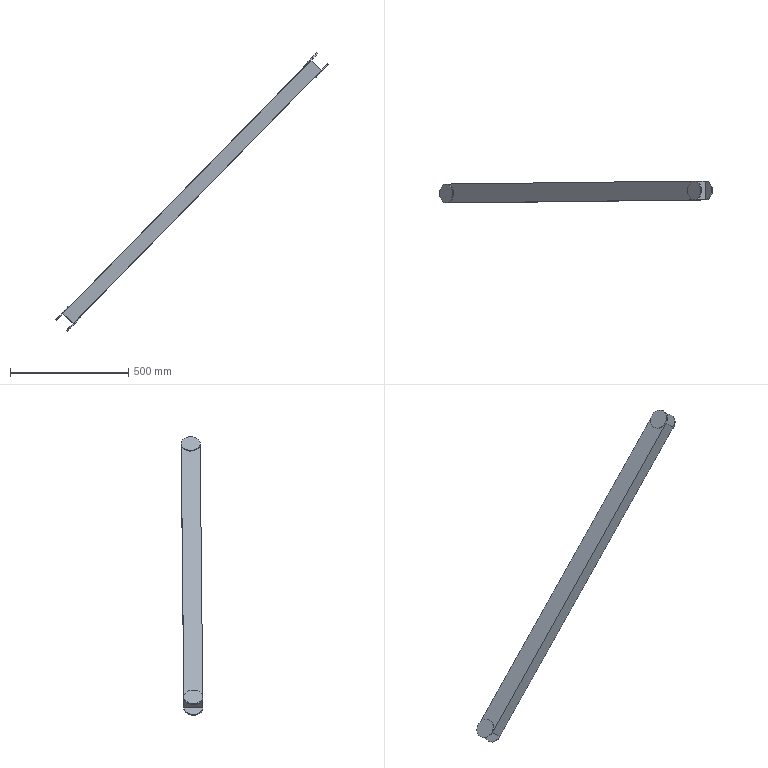Part | SolidWorks | features BaseBody 1 | 1 solid | 22 faces | box 1155 x 90.969 x 1178 mm | volume 7300531 mm3 | plane 14 | cylinder 8 | commonest cylinder face diameters 80 x8
STEP:
#1=CARTESIAN_POINT('',(-1102.13,1023.231,-2093.038));
#2=VERTEX_POINT('',#1);
#3=CARTESIAN_POINT('',(-1046.174,1023.231,-2035.863));
#4=VERTEX_POINT('',#3);
#5=CARTESIAN_POINT('',(-1074.152,1023.231,-2064.451));
#6=DIRECTION('',(0.7147,0.,-0.6994));
#7=DIRECTION('',(-0.6994,0.,-0.7147));
#8=AXIS2_PLACEMENT_3D('',#5,#6,#7);
#9=CIRCLE('',#8,40.);
#10=EDGE_CURVE('',#2,#4,#9,.T.);
#11=ORIENTED_EDGE('',*,*,#10,.T.);
#12=CARTESIAN_POINT('',(-1042.601,1023.231,-2039.36));
#13=VERTEX_POINT('',#12);
#14=CARTESIAN_POINT('',(-1046.174,1023.231,-2035.863));
#15=DIRECTION('',(0.7147,0.,-0.6994));
#16=VECTOR('',#15,1000.);
#17=LINE('',#14,#16);
#18=EDGE_CURVE('',#4,#13,#17,.T.);
#19=ORIENTED_EDGE('',*,*,#18,.T.);
#20=CARTESIAN_POINT('',(-1070.783,1063.23,-2068.157));
#21=VERTEX_POINT('',#20);
#22=CARTESIAN_POINT('',(-1070.579,1023.231,-2067.948));
#23=DIRECTION('',(-0.7147,0.,0.6994));
#24=DIRECTION('',(-0.6994,0.,-0.7147));
#25=AXIS2_PLACEMENT_3D('',#22,#23,#24);
#26=CIRCLE('',#25,40.);
#27=EDGE_CURVE('',#13,#21,#26,.T.);
#28=ORIENTED_EDGE('',*,*,#27,.T.);
#29=CARTESIAN_POINT('',(-1098.556,1023.231,-2096.535));
#30=VERTEX_POINT('',#29);
#31=CARTESIAN_POINT('',(-1070.579,1023.231,-2067.948));
#32=DIRECTION('',(-0.7147,0.,0.6994));
#33=DIRECTION('',(-0.6994,0.,-0.7147));
#34=AXIS2_PLACEMENT_3D('',#31,#32,#33);
#35=CIRCLE('',#34,40.);
#36=EDGE_CURVE('',#21,#30,#35,.T.);
#37=ORIENTED_EDGE('',*,*,#36,.T.);
#38=CARTESIAN_POINT('',(-1102.13,1023.231,-2093.038));
#39=DIRECTION('',(0.7147,0.,-0.6994));
#40=VECTOR('',#39,1000.);
#41=LINE('',#38,#40);
#42=EDGE_CURVE('',#2,#30,#41,.T.);
#43=ORIENTED_EDGE('',*,*,#42,.F.);
#44=EDGE_LOOP('',(#11,#19,#28,#37,#43));
#45=FACE_OUTER_BOUND('',#44,.T.);
#46=CARTESIAN_POINT('',(-1074.152,1023.231,-2064.451));
#47=DIRECTION('',(0.7147,0.,-0.6994));
#48=DIRECTION('',(-0.6994,0.,-0.7147));
#49=AXIS2_PLACEMENT_3D('',#46,#47,#48);
#50=CYLINDRICAL_SURFACE('',#49,40.);
#51=ADVANCED_FACE('',(#45),#50,.T.);
#52=CARTESIAN_POINT('',(-52.992,1034.2,-1021.036));
#53=VERTEX_POINT('',#52);
#54=CARTESIAN_POINT('',(2.964,1034.2,-963.861));
#55=VERTEX_POINT('',#54);
#56=CARTESIAN_POINT('',(-25.014,1034.2,-992.448));
#57=DIRECTION('',(0.7147,0.,-0.6994));
#58=DIRECTION('',(-0.6994,0.,-0.7147));
#59=AXIS2_PLACEMENT_3D('',#56,#57,#58);
#60=CIRCLE('',#59,40.);
#61=EDGE_CURVE('',#53,#55,#60,.T.);
#62=ORIENTED_EDGE('',*,*,#61,.T.);
#63=CARTESIAN_POINT('',(6.537,1034.2,-967.358));
#64=VERTEX_POINT('',#63);
#65=CARTESIAN_POINT('',(2.964,1034.2,-963.861));
#66=DIRECTION('',(0.7147,0.,-0.6994));
#67=VECTOR('',#66,1000.);
#68=LINE('',#65,#67);
#69=EDGE_CURVE('',#55,#64,#68,.T.);
#70=ORIENTED_EDGE('',*,*,#69,.T.);
#71=CARTESIAN_POINT('',(-21.645,1074.199,-996.154));
#72=VERTEX_POINT('',#71);
#73=CARTESIAN_POINT('',(-21.441,1034.2,-995.945));
#74=DIRECTION('',(-0.7147,0.,0.6994));
#75=DIRECTION('',(-0.6994,0.,-0.7147));
#76=AXIS2_PLACEMENT_3D('',#73,#74,#75);
#77=CIRCLE('',#76,40.);
#78=EDGE_CURVE('',#64,#72,#77,.T.);
#79=ORIENTED_EDGE('',*,*,#78,.T.);
#80=CARTESIAN_POINT('',(-49.418,1034.2,-1024.533));
#81=VERTEX_POINT('',#80);
#82=CARTESIAN_POINT('',(-21.441,1034.2,-995.945));
#83=DIRECTION('',(-0.7147,0.,0.6994));
#84=DIRECTION('',(-0.6994,0.,-0.7147));
#85=AXIS2_PLACEMENT_3D('',#82,#83,#84);
#86=CIRCLE('',#85,40.);
#87=EDGE_CURVE('',#72,#81,#86,.T.);
#88=ORIENTED_EDGE('',*,*,#87,.T.);
#89=CARTESIAN_POINT('',(-52.992,1034.2,-1021.036));
#90=DIRECTION('',(0.7147,0.,-0.6994));
#91=VECTOR('',#90,1000.);
#92=LINE('',#89,#91);
#93=EDGE_CURVE('',#53,#81,#92,.T.);
#94=ORIENTED_EDGE('',*,*,#93,.F.);
#95=EDGE_LOOP('',(#62,#70,#79,#88,#94));
#96=FACE_OUTER_BOUND('',#95,.T.);
#97=CARTESIAN_POINT('',(-25.014,1034.2,-992.448));
#98=DIRECTION('',(0.7147,0.,-0.6994));
#99=DIRECTION('',(-0.6994,0.,-0.7147));
#100=AXIS2_PLACEMENT_3D('',#97,#98,#99);
#101=CYLINDRICAL_SURFACE('',#100,40.);
#102=ADVANCED_FACE('',(#96),#101,.T.);
#103=CARTESIAN_POINT('',(-996.146,1023.231,-2084.824));
#104=VERTEX_POINT('',#103);
#105=CARTESIAN_POINT('',(-1052.102,1023.231,-2141.999));
#106=VERTEX_POINT('',#105);
#107=CARTESIAN_POINT('',(-1024.124,1023.231,-2113.412));
#108=DIRECTION('',(-0.7147,0.,0.6994));
#109=DIRECTION('',(0.6994,0.,0.7147));
#110=AXIS2_PLACEMENT_3D('',#107,#108,#109);
#111=CIRCLE('',#110,40.);
#112=EDGE_CURVE('',#104,#106,#111,.T.);
#113=ORIENTED_EDGE('',*,*,#112,.T.);
#114=CARTESIAN_POINT('',(-1055.675,1023.231,-2138.502));
#115=VERTEX_POINT('',#114);
#116=CARTESIAN_POINT('',(-1052.102,1023.231,-2141.999));
#117=DIRECTION('',(-0.7147,0.,0.6994));
#118=VECTOR('',#117,1000.);
#119=LINE('',#116,#118);
#120=EDGE_CURVE('',#106,#115,#119,.T.);
#121=ORIENTED_EDGE('',*,*,#120,.T.);
#122=CARTESIAN_POINT('',(-1027.902,1063.23,-2110.124));
#123=VERTEX_POINT('',#122);
#124=CARTESIAN_POINT('',(-1027.697,1023.231,-2109.915));
#125=DIRECTION('',(0.7147,0.,-0.6994));
#126=DIRECTION('',(0.6994,0.,0.7147));
#127=AXIS2_PLACEMENT_3D('',#124,#125,#126);
#128=CIRCLE('',#127,40.);
#129=EDGE_CURVE('',#115,#123,#128,.T.);
#130=ORIENTED_EDGE('',*,*,#129,.T.);
#131=CARTESIAN_POINT('',(-999.72,1023.231,-2081.327));
#132=VERTEX_POINT('',#131);
#133=CARTESIAN_POINT('',(-1027.697,1023.231,-2109.915));
#134=DIRECTION('',(0.7147,0.,-0.6994));
#135=DIRECTION('',(0.6994,0.,0.7147));
#136=AXIS2_PLACEMENT_3D('',#133,#134,#135);
#137=CIRCLE('',#136,40.);
#138=EDGE_CURVE('',#123,#132,#137,.T.);
#139=ORIENTED_EDGE('',*,*,#138,.T.);
#140=CARTESIAN_POINT('',(-996.146,1023.231,-2084.824));
#141=DIRECTION('',(-0.7147,0.,0.6994));
#142=VECTOR('',#141,1000.);
#143=LINE('',#140,#142);
#144=EDGE_CURVE('',#104,#132,#143,.T.);
#145=ORIENTED_EDGE('',*,*,#144,.F.);
#146=EDGE_LOOP('',(#113,#121,#130,#139,#145));
#147=FACE_OUTER_BOUND('',#146,.T.);
#148=CARTESIAN_POINT('',(-1024.124,1023.231,-2113.412));
#149=DIRECTION('',(-0.7147,0.,0.6994));
#150=DIRECTION('',(0.6994,0.,0.7147));
#151=AXIS2_PLACEMENT_3D('',#148,#149,#150);
#152=CYLINDRICAL_SURFACE('',#151,40.);
#153=ADVANCED_FACE('',(#147),#152,.T.);
#154=CARTESIAN_POINT('',(52.992,1034.2,-1012.822));
#155=VERTEX_POINT('',#154);
#156=CARTESIAN_POINT('',(-2.964,1034.2,-1069.997));
#157=VERTEX_POINT('',#156);
#158=CARTESIAN_POINT('',(25.014,1034.2,-1041.409));
#159=DIRECTION('',(-0.7147,0.,0.6994));
#160=DIRECTION('',(0.6994,0.,0.7147));
#161=AXIS2_PLACEMENT_3D('',#158,#159,#160);
#162=CIRCLE('',#161,40.);
#163=EDGE_CURVE('',#155,#157,#162,.T.);
#164=ORIENTED_EDGE('',*,*,#163,.T.);
#165=CARTESIAN_POINT('',(-6.537,1034.2,-1066.5));
#166=VERTEX_POINT('',#165);
#167=CARTESIAN_POINT('',(-2.964,1034.2,-1069.997));
#168=DIRECTION('',(-0.7147,0.,0.6994));
#169=VECTOR('',#168,1000.);
#170=LINE('',#167,#169);
#171=EDGE_CURVE('',#157,#166,#170,.T.);
#172=ORIENTED_EDGE('',*,*,#171,.T.);
#173=CARTESIAN_POINT('',(21.236,1074.199,-1038.121));
#174=VERTEX_POINT('',#173);
#175=CARTESIAN_POINT('',(21.441,1034.2,-1037.912));
#176=DIRECTION('',(0.7147,0.,-0.6994));
#177=DIRECTION('',(0.6994,0.,0.7147));
#178=AXIS2_PLACEMENT_3D('',#175,#176,#177);
#179=CIRCLE('',#178,40.);
#180=EDGE_CURVE('',#166,#174,#179,.T.);
#181=ORIENTED_EDGE('',*,*,#180,.T.);
#182=CARTESIAN_POINT('',(49.418,1034.2,-1009.325));
#183=VERTEX_POINT('',#182);
#184=CARTESIAN_POINT('',(21.441,1034.2,-1037.912));
#185=DIRECTION('',(0.7147,0.,-0.6994));
#186=DIRECTION('',(0.6994,0.,0.7147));
#187=AXIS2_PLACEMENT_3D('',#184,#185,#186);
#188=CIRCLE('',#187,40.);
#189=EDGE_CURVE('',#174,#183,#188,.T.);
#190=ORIENTED_EDGE('',*,*,#189,.T.);
#191=CARTESIAN_POINT('',(52.992,1034.2,-1012.822));
#192=DIRECTION('',(-0.7147,0.,0.6994));
#193=VECTOR('',#192,1000.);
#194=LINE('',#191,#193);
#195=EDGE_CURVE('',#155,#183,#194,.T.);
#196=ORIENTED_EDGE('',*,*,#195,.F.);
#197=EDGE_LOOP('',(#164,#172,#181,#190,#196));
#198=FACE_OUTER_BOUND('',#197,.T.);
#199=CARTESIAN_POINT('',(25.014,1034.2,-1041.409));
#200=DIRECTION('',(-0.7147,0.,0.6994));
#201=DIRECTION('',(0.6994,0.,0.7147));
#202=AXIS2_PLACEMENT_3D('',#199,#200,#201);
#203=CYLINDRICAL_SURFACE('',#202,40.);
#204=ADVANCED_FACE('',(#198),#203,.T.);
#205=CARTESIAN_POINT('',(-21.236,994.201,-995.736));
#206=VERTEX_POINT('',#205);
#207=CARTESIAN_POINT('',(-1070.374,983.232,-2067.739));
#208=VERTEX_POINT('',#207);
#209=CARTESIAN_POINT('',(-21.236,994.201,-995.736));
#210=DIRECTION('',(-0.6994,-0.007312,-0.7147));
#211=VECTOR('',#210,1000.);
#212=LINE('',#209,#211);
#213=EDGE_CURVE('',#206,#208,#212,.T.);
#214=ORIENTED_EDGE('',*,*,#213,.F.);
#215=CARTESIAN_POINT('',(-21.441,1034.2,-995.945));
#216=DIRECTION('',(-0.7147,0.,0.6994));
#217=DIRECTION('',(-0.6994,0.,-0.7147));
#218=AXIS2_PLACEMENT_3D('',#215,#216,#217);
#219=CIRCLE('',#218,40.);
#220=EDGE_CURVE('',#81,#206,#219,.T.);
#221=ORIENTED_EDGE('',*,*,#220,.F.);
#222=ORIENTED_EDGE('',*,*,#87,.F.);
#223=CARTESIAN_POINT('',(-1070.783,1063.23,-2068.157));
#224=DIRECTION('',(0.6994,0.007312,0.7147));
#225=VECTOR('',#224,1000.);
#226=LINE('',#223,#225);
#227=EDGE_CURVE('',#21,#72,#226,.T.);
#228=ORIENTED_EDGE('',*,*,#227,.F.);
#229=ORIENTED_EDGE('',*,*,#27,.F.);
#230=CARTESIAN_POINT('',(-1070.579,1023.231,-2067.948));
#231=DIRECTION('',(-0.7147,0.,0.6994));
#232=DIRECTION('',(-0.6994,0.,-0.7147));
#233=AXIS2_PLACEMENT_3D('',#230,#231,#232);
#234=CIRCLE('',#233,40.);
#235=EDGE_CURVE('',#208,#13,#234,.T.);
#236=ORIENTED_EDGE('',*,*,#235,.F.);
#237=EDGE_LOOP('',(#214,#221,#222,#228,#229,#236));
#238=FACE_OUTER_BOUND('',#237,.T.);
#239=CARTESIAN_POINT('',(-1070.374,983.232,-2067.739));
#240=DIRECTION('',(0.7147,0.,-0.6994));
#241=DIRECTION('',(-0.6994,0.,-0.7147));
#242=AXIS2_PLACEMENT_3D('',#239,#240,#241);
#243=PLANE('',#242);
#244=ADVANCED_FACE('',(#238),#243,.F.);
#245=ORIENTED_EDGE('',*,*,#18,.F.);
#246=CARTESIAN_POINT('',(-1074.152,1023.231,-2064.451));
#247=DIRECTION('',(0.7147,0.,-0.6994));
#248=DIRECTION('',(-0.6994,0.,-0.7147));
#249=AXIS2_PLACEMENT_3D('',#246,#247,#248);
#250=CIRCLE('',#249,40.);
#251=EDGE_CURVE('',#4,#2,#250,.T.);
#252=ORIENTED_EDGE('',*,*,#251,.T.);
#253=ORIENTED_EDGE('',*,*,#42,.T.);
#254=CARTESIAN_POINT('',(-1070.579,1023.231,-2067.948));
#255=DIRECTION('',(-0.7147,0.,0.6994));
#256=DIRECTION('',(-0.6994,0.,-0.7147));
#257=AXIS2_PLACEMENT_3D('',#254,#255,#256);
#258=CIRCLE('',#257,40.);
#259=EDGE_CURVE('',#30,#208,#258,.T.);
#260=ORIENTED_EDGE('',*,*,#259,.T.);
#261=ORIENTED_EDGE('',*,*,#235,.T.);
#262=EDGE_LOOP('',(#245,#252,#253,#260,#261));
#263=FACE_OUTER_BOUND('',#262,.T.);
#264=CARTESIAN_POINT('',(-1074.152,1023.231,-2064.451));
#265=DIRECTION('',(0.7147,0.,-0.6994));
#266=DIRECTION('',(-0.6994,0.,-0.7147));
#267=AXIS2_PLACEMENT_3D('',#264,#265,#266);
#268=CYLINDRICAL_SURFACE('',#267,40.);
#269=ADVANCED_FACE('',(#263),#268,.T.);
#270=ORIENTED_EDGE('',*,*,#213,.T.);
#271=CARTESIAN_POINT('',(-1027.493,983.232,-2109.705));
#272=VERTEX_POINT('',#271);
#273=CARTESIAN_POINT('',(-1027.493,983.232,-2109.705));
#274=DIRECTION('',(-0.7147,0.,0.6994));
#275=VECTOR('',#274,1000.);
#276=LINE('',#273,#275);
#277=EDGE_CURVE('',#272,#208,#276,.T.);
#278=ORIENTED_EDGE('',*,*,#277,.F.);
#279=CARTESIAN_POINT('',(21.645,994.201,-1037.703));
#280=VERTEX_POINT('',#279);
#281=CARTESIAN_POINT('',(21.645,994.201,-1037.703));
#282=DIRECTION('',(-0.6994,-0.007312,-0.7147));
#283=VECTOR('',#282,1000.);
#284=LINE('',#281,#283);
#285=EDGE_CURVE('',#280,#272,#284,.T.);
#286=ORIENTED_EDGE('',*,*,#285,.F.);
#287=CARTESIAN_POINT('',(-21.236,994.201,-995.736));
#288=DIRECTION('',(0.7147,0.,-0.6994));
#289=VECTOR('',#288,1000.);
#290=LINE('',#287,#289);
#291=EDGE_CURVE('',#206,#280,#290,.T.);
#292=ORIENTED_EDGE('',*,*,#291,.F.);
#293=EDGE_LOOP('',(#270,#278,#286,#292));
#294=FACE_OUTER_BOUND('',#293,.T.);
#295=CARTESIAN_POINT('',(-1027.493,983.232,-2109.705));
#296=DIRECTION('',(-0.005115,1.,-0.005226));
#297=DIRECTION('',(0.,0.005226,1.));
#298=AXIS2_PLACEMENT_3D('',#295,#296,#297);
#299=PLANE('',#298);
#300=ADVANCED_FACE('',(#294),#299,.F.);
#301=ORIENTED_EDGE('',*,*,#69,.F.);
#302=CARTESIAN_POINT('',(-25.014,1034.2,-992.448));
#303=DIRECTION('',(0.7147,0.,-0.6994));
#304=DIRECTION('',(-0.6994,0.,-0.7147));
#305=AXIS2_PLACEMENT_3D('',#302,#303,#304);
#306=CIRCLE('',#305,40.);
#307=EDGE_CURVE('',#55,#53,#306,.T.);
#308=ORIENTED_EDGE('',*,*,#307,.T.);
#309=ORIENTED_EDGE('',*,*,#93,.T.);
#310=ORIENTED_EDGE('',*,*,#220,.T.);
#311=CARTESIAN_POINT('',(-21.441,1034.2,-995.945));
#312=DIRECTION('',(-0.7147,0.,0.6994));
#313=DIRECTION('',(-0.6994,0.,-0.7147));
#314=AXIS2_PLACEMENT_3D('',#311,#312,#313);
#315=CIRCLE('',#314,40.);
#316=EDGE_CURVE('',#206,#64,#315,.T.);
#317=ORIENTED_EDGE('',*,*,#316,.T.);
#318=EDGE_LOOP('',(#301,#308,#309,#310,#317));
#319=FACE_OUTER_BOUND('',#318,.T.);
#320=CARTESIAN_POINT('',(-25.014,1034.2,-992.448));
#321=DIRECTION('',(0.7147,0.,-0.6994));
#322=DIRECTION('',(-0.6994,0.,-0.7147));
#323=AXIS2_PLACEMENT_3D('',#320,#321,#322);
#324=CYLINDRICAL_SURFACE('',#323,40.);
#325=ADVANCED_FACE('',(#319),#324,.T.);
#326=CARTESIAN_POINT('',(-1027.902,1063.23,-2110.124));
#327=DIRECTION('',(0.6994,0.007312,0.7147));
#328=VECTOR('',#327,1000.);
#329=LINE('',#326,#328);
#330=EDGE_CURVE('',#123,#174,#329,.T.);
#331=ORIENTED_EDGE('',*,*,#330,.F.);
#332=CARTESIAN_POINT('',(-1070.783,1063.23,-2068.157));
#333=DIRECTION('',(0.7147,0.,-0.6994));
#334=VECTOR('',#333,1000.);
#335=LINE('',#332,#334);
#336=EDGE_CURVE('',#21,#123,#335,.T.);
#337=ORIENTED_EDGE('',*,*,#336,.F.);
#338=ORIENTED_EDGE('',*,*,#227,.T.);
#339=CARTESIAN_POINT('',(21.236,1074.199,-1038.121));
#340=DIRECTION('',(-0.7147,0.,0.6994));
#341=VECTOR('',#340,1000.);
#342=LINE('',#339,#341);
#343=EDGE_CURVE('',#174,#72,#342,.T.);
#344=ORIENTED_EDGE('',*,*,#343,.F.);
#345=EDGE_LOOP('',(#331,#337,#338,#344));
#346=FACE_OUTER_BOUND('',#345,.T.);
#347=CARTESIAN_POINT('',(-1027.902,1063.23,-2110.124));
#348=DIRECTION('',(0.005115,-1.,0.005226));
#349=DIRECTION('',(0.,-0.005226,-1.));
#350=AXIS2_PLACEMENT_3D('',#347,#348,#349);
#351=PLANE('',#350);
#352=ADVANCED_FACE('',(#346),#351,.F.);
#353=ORIENTED_EDGE('',*,*,#10,.F.);
#354=ORIENTED_EDGE('',*,*,#251,.F.);
#355=EDGE_LOOP('',(#353,#354));
#356=FACE_OUTER_BOUND('',#355,.T.);
#357=CARTESIAN_POINT('',(-1074.152,1023.231,-2064.451));
#358=DIRECTION('',(-0.7147,0.,0.6994));
#359=DIRECTION('',(0.6994,0.,0.7147));
#360=AXIS2_PLACEMENT_3D('',#357,#358,#359);
#361=PLANE('',#360);
#362=ADVANCED_FACE('',(#356),#361,.T.);
#363=CARTESIAN_POINT('',(21.441,1034.2,-1037.912));
#364=DIRECTION('',(0.005115,-1.,0.005226));
#365=VECTOR('',#364,1000.);
#366=LINE('',#363,#365);
#367=EDGE_CURVE('',#174,#280,#366,.T.);
#368=ORIENTED_EDGE('',*,*,#367,.F.);
#369=ORIENTED_EDGE('',*,*,#343,.T.);
#370=CARTESIAN_POINT('',(-21.441,1034.2,-995.945));
#371=DIRECTION('',(-0.005115,1.,-0.005226));
#372=VECTOR('',#371,1000.);
#373=LINE('',#370,#372);
#374=EDGE_CURVE('',#206,#72,#373,.T.);
#375=ORIENTED_EDGE('',*,*,#374,.F.);
#376=ORIENTED_EDGE('',*,*,#291,.T.);
#377=EDGE_LOOP('',(#368,#369,#375,#376));
#378=FACE_OUTER_BOUND('',#377,.T.);
#379=CARTESIAN_POINT('',(0.,1034.2,-1016.929));
#380=DIRECTION('',(-0.6994,-0.007312,-0.7147));
#381=DIRECTION('',(-0.7147,0.,0.6994));
#382=AXIS2_PLACEMENT_3D('',#379,#380,#381);
#383=PLANE('',#382);
#384=ADVANCED_FACE('',(#378),#383,.F.);
#385=ORIENTED_EDGE('',*,*,#336,.T.);
#386=CARTESIAN_POINT('',(-1027.697,1023.231,-2109.915));
#387=DIRECTION('',(0.005115,-1.,0.005226));
#388=VECTOR('',#387,1000.);
#389=LINE('',#386,#388);
#390=EDGE_CURVE('',#123,#272,#389,.T.);
#391=ORIENTED_EDGE('',*,*,#390,.T.);
#392=ORIENTED_EDGE('',*,*,#277,.T.);
#393=CARTESIAN_POINT('',(-1070.579,1023.231,-2067.948));
#394=DIRECTION('',(-0.005115,1.,-0.005226));
#395=VECTOR('',#394,1000.);
#396=LINE('',#393,#395);
#397=EDGE_CURVE('',#208,#21,#396,.T.);
#398=ORIENTED_EDGE('',*,*,#397,.T.);
#399=EDGE_LOOP('',(#385,#391,#392,#398));
#400=FACE_OUTER_BOUND('',#399,.T.);
#401=CARTESIAN_POINT('',(-1049.138,1023.231,-2088.931));
#402=DIRECTION('',(-0.6994,-0.007312,-0.7147));
#403=DIRECTION('',(-0.7147,0.,0.6994));
#404=AXIS2_PLACEMENT_3D('',#401,#402,#403);
#405=PLANE('',#404);
#406=ADVANCED_FACE('',(#400),#405,.T.);
#407=ORIENTED_EDGE('',*,*,#330,.T.);
#408=ORIENTED_EDGE('',*,*,#180,.F.);
#409=CARTESIAN_POINT('',(21.441,1034.2,-1037.912));
#410=DIRECTION('',(0.7147,0.,-0.6994));
#411=DIRECTION('',(0.6994,0.,0.7147));
#412=AXIS2_PLACEMENT_3D('',#409,#410,#411);
#413=CIRCLE('',#412,40.);
#414=EDGE_CURVE('',#280,#166,#413,.T.);
#415=ORIENTED_EDGE('',*,*,#414,.F.);
#416=ORIENTED_EDGE('',*,*,#285,.T.);
#417=CARTESIAN_POINT('',(-1027.697,1023.231,-2109.915));
#418=DIRECTION('',(0.7147,0.,-0.6994));
#419=DIRECTION('',(0.6994,0.,0.7147));
#420=AXIS2_PLACEMENT_3D('',#417,#418,#419);
#421=CIRCLE('',#420,40.);
#422=EDGE_CURVE('',#132,#272,#421,.T.);
#423=ORIENTED_EDGE('',*,*,#422,.F.);
#424=ORIENTED_EDGE('',*,*,#138,.F.);
#425=EDGE_LOOP('',(#407,#408,#415,#416,#423,#424));
#426=FACE_OUTER_BOUND('',#425,.T.);
#427=CARTESIAN_POINT('',(-1027.493,983.232,-2109.705));
#428=DIRECTION('',(-0.7147,0.,0.6994));
#429=DIRECTION('',(0.6994,0.,0.7147));
#430=AXIS2_PLACEMENT_3D('',#427,#428,#429);
#431=PLANE('',#430);
#432=ADVANCED_FACE('',(#426),#431,.F.);
#433=ORIENTED_EDGE('',*,*,#61,.F.);
#434=ORIENTED_EDGE('',*,*,#307,.F.);
#435=EDGE_LOOP('',(#433,#434));
#436=FACE_OUTER_BOUND('',#435,.T.);
#437=CARTESIAN_POINT('',(-25.014,1034.2,-992.448));
#438=DIRECTION('',(-0.7147,0.,0.6994));
#439=DIRECTION('',(0.6994,0.,0.7147));
#440=AXIS2_PLACEMENT_3D('',#437,#438,#439);
#441=PLANE('',#440);
#442=ADVANCED_FACE('',(#436),#441,.T.);
#443=ORIENTED_EDGE('',*,*,#36,.F.);
#444=ORIENTED_EDGE('',*,*,#397,.F.);
#445=ORIENTED_EDGE('',*,*,#259,.F.);
#446=EDGE_LOOP('',(#443,#444,#445));
#447=FACE_OUTER_BOUND('',#446,.T.);
#448=CARTESIAN_POINT('',(-1070.579,1023.231,-2067.948));
#449=DIRECTION('',(-0.7147,0.,0.6994));
#450=DIRECTION('',(0.6994,0.,0.7147));
#451=AXIS2_PLACEMENT_3D('',#448,#449,#450);
#452=PLANE('',#451);
#453=ADVANCED_FACE('',(#447),#452,.F.);
#454=ORIENTED_EDGE('',*,*,#367,.T.);
#455=CARTESIAN_POINT('',(21.441,1034.2,-1037.912));
#456=DIRECTION('',(0.7147,0.,-0.6994));
#457=DIRECTION('',(0.6994,0.,0.7147));
#458=AXIS2_PLACEMENT_3D('',#455,#456,#457);
#459=CIRCLE('',#458,40.);
#460=EDGE_CURVE('',#183,#280,#459,.T.);
#461=ORIENTED_EDGE('',*,*,#460,.F.);
#462=ORIENTED_EDGE('',*,*,#189,.F.);
#463=EDGE_LOOP('',(#454,#461,#462));
#464=FACE_OUTER_BOUND('',#463,.T.);
#465=CARTESIAN_POINT('',(21.441,1034.2,-1037.912));
#466=DIRECTION('',(0.7147,0.,-0.6994));
#467=DIRECTION('',(-0.6994,0.,-0.7147));
#468=AXIS2_PLACEMENT_3D('',#465,#466,#467);
#469=PLANE('',#468);
#470=ADVANCED_FACE('',(#464),#469,.F.);
#471=ORIENTED_EDGE('',*,*,#374,.T.);
#472=ORIENTED_EDGE('',*,*,#78,.F.);
#473=ORIENTED_EDGE('',*,*,#316,.F.);
#474=EDGE_LOOP('',(#471,#472,#473));
#475=FACE_OUTER_BOUND('',#474,.T.);
#476=CARTESIAN_POINT('',(-21.441,1034.2,-995.945));
#477=DIRECTION('',(-0.7147,0.,0.6994));
#478=DIRECTION('',(0.6994,0.,0.7147));
#479=AXIS2_PLACEMENT_3D('',#476,#477,#478);
#480=PLANE('',#479);
#481=ADVANCED_FACE('',(#475),#480,.F.);
#482=CARTESIAN_POINT('',(-1027.697,1023.231,-2109.915));
#483=DIRECTION('',(0.7147,0.,-0.6994));
#484=DIRECTION('',(0.6994,0.,0.7147));
#485=AXIS2_PLACEMENT_3D('',#482,#483,#484);
#486=CIRCLE('',#485,40.);
#487=EDGE_CURVE('',#272,#115,#486,.T.);
#488=ORIENTED_EDGE('',*,*,#487,.F.);
#489=ORIENTED_EDGE('',*,*,#390,.F.);
#490=ORIENTED_EDGE('',*,*,#129,.F.);
#491=EDGE_LOOP('',(#488,#489,#490));
#492=FACE_OUTER_BOUND('',#491,.T.);
#493=CARTESIAN_POINT('',(-1027.697,1023.231,-2109.915));
#494=DIRECTION('',(0.7147,0.,-0.6994));
#495=DIRECTION('',(-0.6994,0.,-0.7147));
#496=AXIS2_PLACEMENT_3D('',#493,#494,#495);
#497=PLANE('',#496);
#498=ADVANCED_FACE('',(#492),#497,.F.);
#499=ORIENTED_EDGE('',*,*,#120,.F.);
#500=CARTESIAN_POINT('',(-1024.124,1023.231,-2113.412));
#501=DIRECTION('',(-0.7147,0.,0.6994));
#502=DIRECTION('',(0.6994,0.,0.7147));
#503=AXIS2_PLACEMENT_3D('',#500,#501,#502);
#504=CIRCLE('',#503,40.);
#505=EDGE_CURVE('',#106,#104,#504,.T.);
#506=ORIENTED_EDGE('',*,*,#505,.T.);
#507=ORIENTED_EDGE('',*,*,#144,.T.);
#508=ORIENTED_EDGE('',*,*,#422,.T.);
#509=ORIENTED_EDGE('',*,*,#487,.T.);
#510=EDGE_LOOP('',(#499,#506,#507,#508,#509));
#511=FACE_OUTER_BOUND('',#510,.T.);
#512=CARTESIAN_POINT('',(-1024.124,1023.231,-2113.412));
#513=DIRECTION('',(-0.7147,0.,0.6994));
#514=DIRECTION('',(0.6994,0.,0.7147));
#515=AXIS2_PLACEMENT_3D('',#512,#513,#514);
#516=CYLINDRICAL_SURFACE('',#515,40.);
#517=ADVANCED_FACE('',(#511),#516,.T.);
#518=ORIENTED_EDGE('',*,*,#171,.F.);
#519=CARTESIAN_POINT('',(25.014,1034.2,-1041.409));
#520=DIRECTION('',(-0.7147,0.,0.6994));
#521=DIRECTION('',(0.6994,0.,0.7147));
#522=AXIS2_PLACEMENT_3D('',#519,#520,#521);
#523=CIRCLE('',#522,40.);
#524=EDGE_CURVE('',#157,#155,#523,.T.);
#525=ORIENTED_EDGE('',*,*,#524,.T.);
#526=ORIENTED_EDGE('',*,*,#195,.T.);
#527=ORIENTED_EDGE('',*,*,#460,.T.);
#528=ORIENTED_EDGE('',*,*,#414,.T.);
#529=EDGE_LOOP('',(#518,#525,#526,#527,#528));
#530=FACE_OUTER_BOUND('',#529,.T.);
#531=CARTESIAN_POINT('',(25.014,1034.2,-1041.409));
#532=DIRECTION('',(-0.7147,0.,0.6994));
#533=DIRECTION('',(0.6994,0.,0.7147));
#534=AXIS2_PLACEMENT_3D('',#531,#532,#533);
#535=CYLINDRICAL_SURFACE('',#534,40.);
#536=ADVANCED_FACE('',(#530),#535,.T.);
#537=ORIENTED_EDGE('',*,*,#112,.F.);
#538=ORIENTED_EDGE('',*,*,#505,.F.);
#539=EDGE_LOOP('',(#537,#538));
#540=FACE_OUTER_BOUND('',#539,.T.);
#541=CARTESIAN_POINT('',(-1024.124,1023.231,-2113.412));
#542=DIRECTION('',(0.7147,0.,-0.6994));
#543=DIRECTION('',(-0.6994,0.,-0.7147));
#544=AXIS2_PLACEMENT_3D('',#541,#542,#543);
#545=PLANE('',#544);
#546=ADVANCED_FACE('',(#540),#545,.T.);
#547=ORIENTED_EDGE('',*,*,#163,.F.);
#548=ORIENTED_EDGE('',*,*,#524,.F.);
#549=EDGE_LOOP('',(#547,#548));
#550=FACE_OUTER_BOUND('',#549,.T.);
#551=CARTESIAN_POINT('',(25.014,1034.2,-1041.409));
#552=DIRECTION('',(0.7147,0.,-0.6994));
#553=DIRECTION('',(-0.6994,0.,-0.7147));
#554=AXIS2_PLACEMENT_3D('',#551,#552,#553);
#555=PLANE('',#554);
#556=ADVANCED_FACE('',(#550),#555,.T.);
#557=CLOSED_SHELL('',(#51,#102,#153,#204,#244,#269,#300,#325,#352,#362,#384,#406,#432,#442,#453,#470,#481,#498,#517,#536,#546,#556));
#558=MANIFOLD_SOLID_BREP('',#557);
#559=CARTESIAN_POINT('',(0.,0.,0.));
#560=DIRECTION('',(0.,0.,1.));
#561=DIRECTION('',(1.,0.,0.));
#562=AXIS2_PLACEMENT_3D('',#559,#560,#561);
#563=(LENGTH_UNIT()NAMED_UNIT(*)SI_UNIT(.MILLI.,.METRE.));
#564=UNCERTAINTY_MEASURE_WITH_UNIT(LENGTH_MEASURE(0.00001),#563,'','');
#565=(NAMED_UNIT(*)PLANE_ANGLE_UNIT()SI_UNIT($,.RADIAN.));
#566=(NAMED_UNIT(*)SI_UNIT($,.STERADIAN.)SOLID_ANGLE_UNIT());
#567=(GEOMETRIC_REPRESENTATION_CONTEXT(3)GLOBAL_UNCERTAINTY_ASSIGNED_CONTEXT((#564))GLOBAL_UNIT_ASSIGNED_CONTEXT((#563,#565,#566))REPRESENTATION_CONTEXT('',''));
#568=ADVANCED_BREP_SHAPE_REPRESENTATION('',(#558,#562),#567);